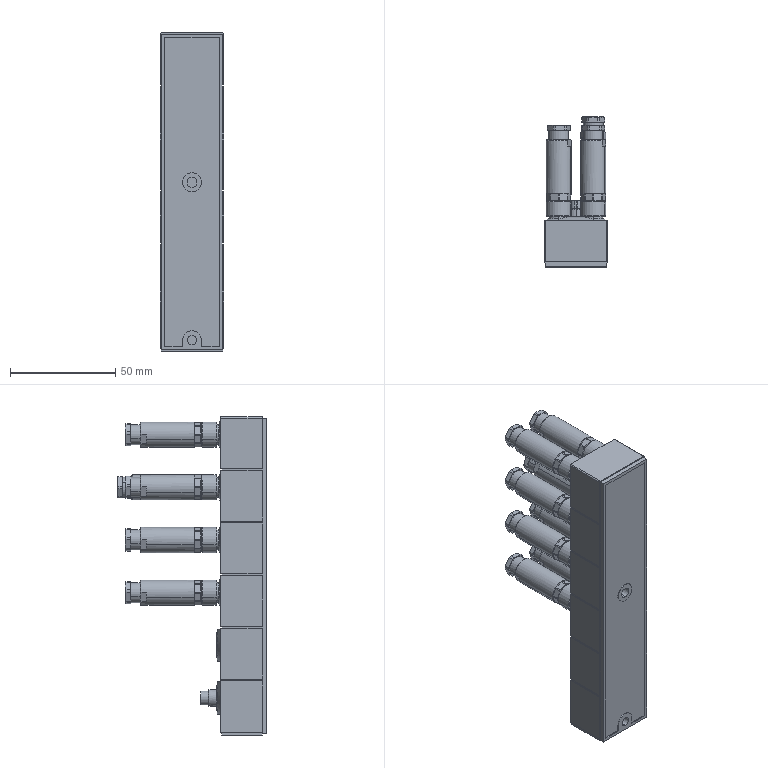Part | SolidWorks | 9 solids | 1123 faces | box 30 x 71.1 x 151 mm | volume 135395 mm3 | plane 459 | cylinder 390 | cone 168 | spline 106 | commonest cylinder face diameters 1 x62 1.03 x48 11 x48 6 x34 12 x32 8 x18